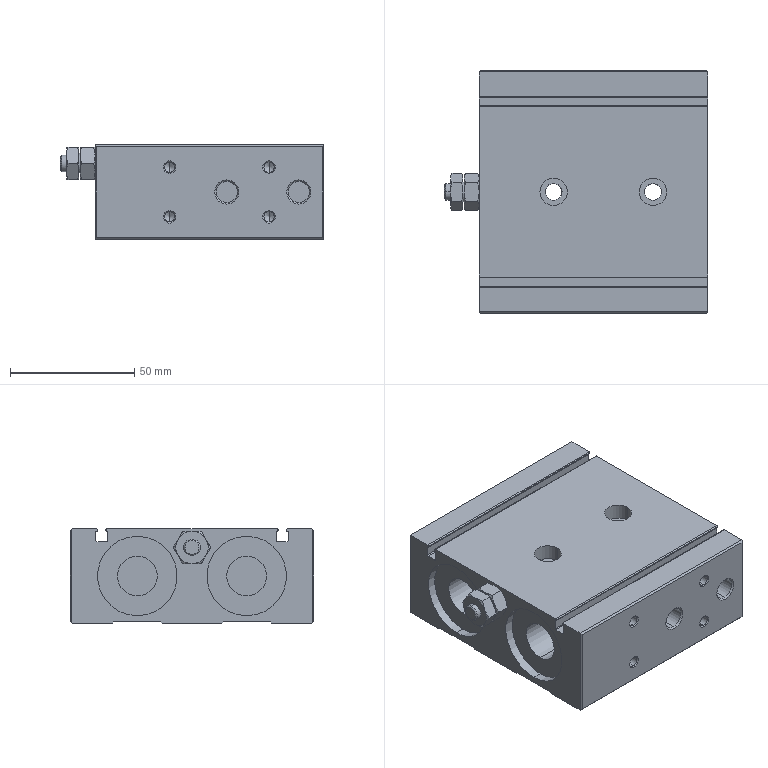Part | STEP file | TR_32x10-1 | 1 solid | 240 faces | box 106 x 98 x 38 mm | volume 251208 mm3 | cylinder 94 | cone 74 | plane 72 | commonest cylinder face diameters 4.134 x16 0.8 x12 6 x12 2.1 x8 8.566 x8 32 x8